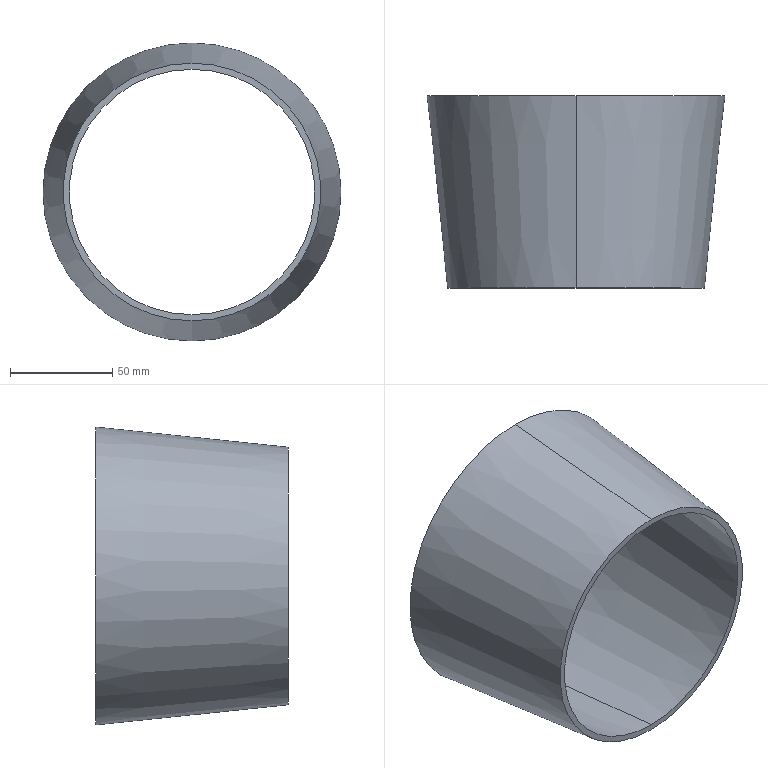Part | STEP file | getao2 | 1 solid | 6 faces | box 146 x 94.195 x 146 mm | volume 118161 mm3 | cone 4 | plane 2
STEP:
#1=CARTESIAN_POINT('',(0.,-137.455,-60.1));
#2=VERTEX_POINT('',#1);
#3=CARTESIAN_POINT('',(0.,-137.455,60.1));
#4=VERTEX_POINT('',#3);
#5=CARTESIAN_POINT('',(0.,-137.455,0.));
#6=DIRECTION('',(0.,1.,0.));
#7=DIRECTION('',(0.,0.,1.));
#8=AXIS2_PLACEMENT_3D('',#5,#6,#7);
#9=CIRCLE('',#8,60.1);
#10=EDGE_CURVE('',#2,#4,#9,.T.);
#11=ORIENTED_EDGE('',*,*,#10,.F.);
#12=CARTESIAN_POINT('',(0.,-43.26,-70.));
#13=VERTEX_POINT('',#12);
#14=CARTESIAN_POINT('',(0.,-43.26,-70.));
#15=DIRECTION('',(0.,0.9945,-0.1045));
#16=VECTOR('',#15,1000.);
#17=LINE('',#14,#16);
#18=EDGE_CURVE('',#2,#13,#17,.T.);
#19=ORIENTED_EDGE('',*,*,#18,.T.);
#20=CARTESIAN_POINT('',(0.,-43.26,70.));
#21=VERTEX_POINT('',#20);
#22=CARTESIAN_POINT('',(0.,-43.26,0.));
#23=DIRECTION('',(0.,1.,0.));
#24=DIRECTION('',(0.,0.,1.));
#25=AXIS2_PLACEMENT_3D('',#22,#23,#24);
#26=CIRCLE('',#25,70.);
#27=EDGE_CURVE('',#13,#21,#26,.T.);
#28=ORIENTED_EDGE('',*,*,#27,.T.);
#29=CARTESIAN_POINT('',(0.,-43.26,70.));
#30=DIRECTION('',(0.,0.9945,0.1045));
#31=VECTOR('',#30,1000.);
#32=LINE('',#29,#31);
#33=EDGE_CURVE('',#4,#21,#32,.T.);
#34=ORIENTED_EDGE('',*,*,#33,.F.);
#35=EDGE_LOOP('',(#11,#19,#28,#34));
#36=FACE_OUTER_BOUND('',#35,.T.);
#37=CARTESIAN_POINT('',(0.,-43.26,0.));
#38=DIRECTION('',(0.,1.,0.));
#39=DIRECTION('',(0.,0.,1.));
#40=AXIS2_PLACEMENT_3D('',#37,#38,#39);
#41=CONICAL_SURFACE('',#40,70.,0.1047);
#42=ADVANCED_FACE('',(#36),#41,.F.);
#43=CARTESIAN_POINT('',(0.,-137.455,63.1));
#44=VERTEX_POINT('',#43);
#45=CARTESIAN_POINT('',(0.,-137.455,-63.1));
#46=VERTEX_POINT('',#45);
#47=CARTESIAN_POINT('',(0.,-137.455,0.));
#48=DIRECTION('',(0.,1.,0.));
#49=DIRECTION('',(0.,0.,1.));
#50=AXIS2_PLACEMENT_3D('',#47,#48,#49);
#51=CIRCLE('',#50,63.1);
#52=EDGE_CURVE('',#44,#46,#51,.T.);
#53=ORIENTED_EDGE('',*,*,#52,.T.);
#54=CARTESIAN_POINT('',(0.,-43.26,-73.));
#55=VERTEX_POINT('',#54);
#56=CARTESIAN_POINT('',(0.,-137.455,-63.1));
#57=DIRECTION('',(0.,0.9945,-0.1045));
#58=VECTOR('',#57,1000.);
#59=LINE('',#56,#58);
#60=EDGE_CURVE('',#46,#55,#59,.T.);
#61=ORIENTED_EDGE('',*,*,#60,.T.);
#62=CARTESIAN_POINT('',(0.,-43.26,73.));
#63=VERTEX_POINT('',#62);
#64=CARTESIAN_POINT('',(0.,-43.26,0.));
#65=DIRECTION('',(0.,1.,0.));
#66=DIRECTION('',(0.,0.,1.));
#67=AXIS2_PLACEMENT_3D('',#64,#65,#66);
#68=CIRCLE('',#67,73.);
#69=EDGE_CURVE('',#63,#55,#68,.T.);
#70=ORIENTED_EDGE('',*,*,#69,.F.);
#71=CARTESIAN_POINT('',(0.,-137.455,63.1));
#72=DIRECTION('',(0.,0.9945,0.1045));
#73=VECTOR('',#72,1000.);
#74=LINE('',#71,#73);
#75=EDGE_CURVE('',#44,#63,#74,.T.);
#76=ORIENTED_EDGE('',*,*,#75,.F.);
#77=EDGE_LOOP('',(#53,#61,#70,#76));
#78=FACE_OUTER_BOUND('',#77,.T.);
#79=CARTESIAN_POINT('',(0.,-137.455,0.));
#80=DIRECTION('',(0.,1.,0.));
#81=DIRECTION('',(0.,0.,1.));
#82=AXIS2_PLACEMENT_3D('',#79,#80,#81);
#83=CONICAL_SURFACE('',#82,63.1,0.1047);
#84=ADVANCED_FACE('',(#78),#83,.T.);
#85=CARTESIAN_POINT('',(0.,-43.26,0.));
#86=DIRECTION('',(0.,1.,0.));
#87=DIRECTION('',(0.,0.,1.));
#88=AXIS2_PLACEMENT_3D('',#85,#86,#87);
#89=CIRCLE('',#88,70.);
#90=EDGE_CURVE('',#21,#13,#89,.T.);
#91=ORIENTED_EDGE('',*,*,#90,.F.);
#92=ORIENTED_EDGE('',*,*,#27,.F.);
#93=EDGE_LOOP('',(#91,#92));
#94=FACE_BOUND('',#93,.T.);
#95=ORIENTED_EDGE('',*,*,#69,.T.);
#96=CARTESIAN_POINT('',(0.,-43.26,0.));
#97=DIRECTION('',(0.,1.,0.));
#98=DIRECTION('',(0.,0.,1.));
#99=AXIS2_PLACEMENT_3D('',#96,#97,#98);
#100=CIRCLE('',#99,73.);
#101=EDGE_CURVE('',#55,#63,#100,.T.);
#102=ORIENTED_EDGE('',*,*,#101,.T.);
#103=EDGE_LOOP('',(#95,#102));
#104=FACE_OUTER_BOUND('',#103,.T.);
#105=CARTESIAN_POINT('',(70.,-43.26,0.));
#106=DIRECTION('',(0.,-1.,0.));
#107=DIRECTION('',(0.,0.,-1.));
#108=AXIS2_PLACEMENT_3D('',#105,#106,#107);
#109=PLANE('',#108);
#110=ADVANCED_FACE('',(#94,#104),#109,.F.);
#111=ORIENTED_EDGE('',*,*,#60,.F.);
#112=CARTESIAN_POINT('',(0.,-137.455,0.));
#113=DIRECTION('',(0.,1.,0.));
#114=DIRECTION('',(0.,0.,1.));
#115=AXIS2_PLACEMENT_3D('',#112,#113,#114);
#116=CIRCLE('',#115,63.1);
#117=EDGE_CURVE('',#46,#44,#116,.T.);
#118=ORIENTED_EDGE('',*,*,#117,.T.);
#119=ORIENTED_EDGE('',*,*,#75,.T.);
#120=ORIENTED_EDGE('',*,*,#101,.F.);
#121=EDGE_LOOP('',(#111,#118,#119,#120));
#122=FACE_OUTER_BOUND('',#121,.T.);
#123=CARTESIAN_POINT('',(0.,-137.455,0.));
#124=DIRECTION('',(0.,1.,0.));
#125=DIRECTION('',(0.,0.,1.));
#126=AXIS2_PLACEMENT_3D('',#123,#124,#125);
#127=CONICAL_SURFACE('',#126,63.1,0.1047);
#128=ADVANCED_FACE('',(#122),#127,.T.);
#129=ORIENTED_EDGE('',*,*,#52,.F.);
#130=ORIENTED_EDGE('',*,*,#117,.F.);
#131=EDGE_LOOP('',(#129,#130));
#132=FACE_OUTER_BOUND('',#131,.T.);
#133=CARTESIAN_POINT('',(0.,-137.455,0.));
#134=DIRECTION('',(0.,1.,0.));
#135=DIRECTION('',(0.,0.,1.));
#136=AXIS2_PLACEMENT_3D('',#133,#134,#135);
#137=CIRCLE('',#136,60.1);
#138=EDGE_CURVE('',#4,#2,#137,.T.);
#139=ORIENTED_EDGE('',*,*,#138,.T.);
#140=ORIENTED_EDGE('',*,*,#10,.T.);
#141=EDGE_LOOP('',(#139,#140));
#142=FACE_BOUND('',#141,.T.);
#143=CARTESIAN_POINT('',(60.1,-137.455,0.));
#144=DIRECTION('',(0.,1.,0.));
#145=DIRECTION('',(0.,0.,1.));
#146=AXIS2_PLACEMENT_3D('',#143,#144,#145);
#147=PLANE('',#146);
#148=ADVANCED_FACE('',(#132,#142),#147,.F.);
#149=ORIENTED_EDGE('',*,*,#18,.F.);
#150=ORIENTED_EDGE('',*,*,#138,.F.);
#151=ORIENTED_EDGE('',*,*,#33,.T.);
#152=ORIENTED_EDGE('',*,*,#90,.T.);
#153=EDGE_LOOP('',(#149,#150,#151,#152));
#154=FACE_OUTER_BOUND('',#153,.T.);
#155=CARTESIAN_POINT('',(0.,-43.26,0.));
#156=DIRECTION('',(0.,1.,0.));
#157=DIRECTION('',(0.,0.,1.));
#158=AXIS2_PLACEMENT_3D('',#155,#156,#157);
#159=CONICAL_SURFACE('',#158,70.,0.1047);
#160=ADVANCED_FACE('',(#154),#159,.F.);
#161=CLOSED_SHELL('',(#42,#84,#110,#128,#148,#160));
#162=MANIFOLD_SOLID_BREP('',#161);
#163=CARTESIAN_POINT('',(0.,0.,0.));
#164=DIRECTION('',(0.,0.,1.));
#165=DIRECTION('',(1.,0.,0.));
#166=AXIS2_PLACEMENT_3D('',#163,#164,#165);
#167=(LENGTH_UNIT()NAMED_UNIT(*)SI_UNIT(.MILLI.,.METRE.));
#168=UNCERTAINTY_MEASURE_WITH_UNIT(LENGTH_MEASURE(0.00001),#167,'','');
#169=(NAMED_UNIT(*)PLANE_ANGLE_UNIT()SI_UNIT($,.RADIAN.));
#170=(NAMED_UNIT(*)SI_UNIT($,.STERADIAN.)SOLID_ANGLE_UNIT());
#171=(GEOMETRIC_REPRESENTATION_CONTEXT(3)GLOBAL_UNCERTAINTY_ASSIGNED_CONTEXT((#168))GLOBAL_UNIT_ASSIGNED_CONTEXT((#167,#169,#170))REPRESENTATION_CONTEXT('',''));
#172=ADVANCED_BREP_SHAPE_REPRESENTATION('',(#162,#166),#171);